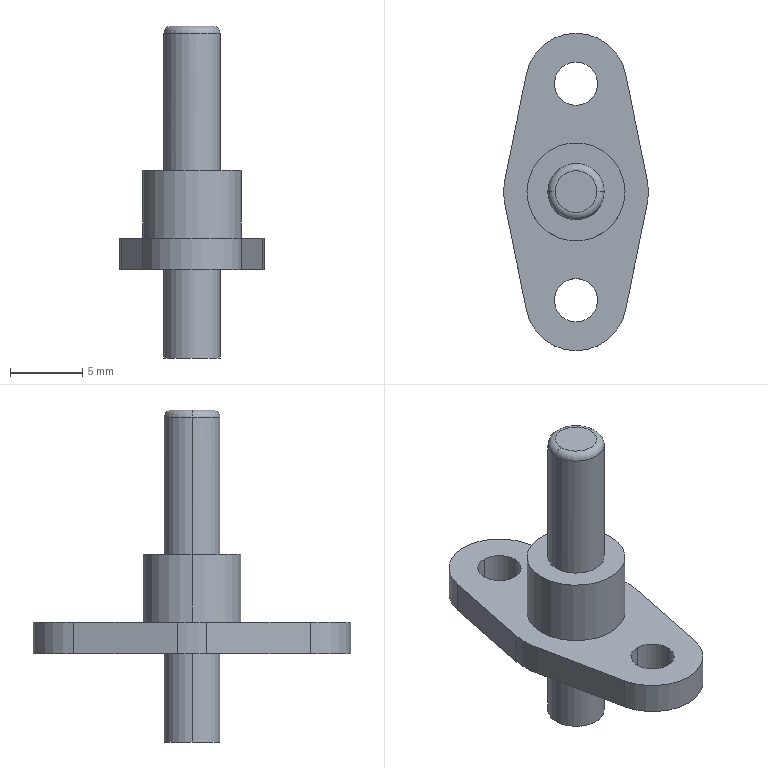Part | STEP file | ZXW722-L-79-1 | 1 solid | 30 faces | box 10 x 22 x 23 mm | volume 593.01 mm3 | cylinder 16 | plane 10 | torus 4 | commonest cylinder face diameters 3 x4 3.9 x4 2.5 x2 6.8 x2 7 x2 10 x2
STEP:
#1=CARTESIAN_POINT('',(0.,0.,0.));
#2=DIRECTION('',(0.,0.,1.));
#3=DIRECTION('',(1.,0.,0.));
#4=AXIS2_PLACEMENT_3D('',#1,#2,#3);
#5=CARTESIAN_POINT('',(1.45,0.,0.));
#6=VERTEX_POINT('',#5);
#7=CARTESIAN_POINT('',(-1.45,0.,0.));
#8=VERTEX_POINT('',#7);
#9=CARTESIAN_POINT('',(0.,0.,0.));
#10=DIRECTION('',(0.,0.,-1.));
#11=DIRECTION('',(1.,0.,0.));
#12=AXIS2_PLACEMENT_3D('',#9,#10,#11);
#13=CIRCLE('',#12,1.45);
#14=EDGE_CURVE('',#6,#8,#13,.T.);
#15=ORIENTED_EDGE('',*,*,#14,.T.);
#16=CARTESIAN_POINT('',(0.,0.,0.));
#17=DIRECTION('',(0.,0.,-1.));
#18=DIRECTION('',(-1.,0.,0.));
#19=AXIS2_PLACEMENT_3D('',#16,#17,#18);
#20=CIRCLE('',#19,1.45);
#21=EDGE_CURVE('',#8,#6,#20,.T.);
#22=ORIENTED_EDGE('',*,*,#21,.T.);
#23=EDGE_LOOP('',(#15,#22));
#24=FACE_OUTER_BOUND('',#23,.F.);
#25=CARTESIAN_POINT('',(0.,0.,0.));
#26=DIRECTION('',(0.,0.,1.));
#27=DIRECTION('',(-1.,0.,0.));
#28=AXIS2_PLACEMENT_3D('',#25,#26,#27);
#29=PLANE('',#28);
#30=ADVANCED_FACE('',(#24),#29,.T.);
#31=CARTESIAN_POINT('',(1.95,0.,-0.5));
#32=VERTEX_POINT('',#31);
#33=CARTESIAN_POINT('',(-1.95,-0.03686,-0.5));
#34=VERTEX_POINT('',#33);
#35=CARTESIAN_POINT('',(0.,0.,-0.5));
#36=DIRECTION('',(0.,0.,-1.));
#37=DIRECTION('',(1.,0.,0.));
#38=AXIS2_PLACEMENT_3D('',#35,#36,#37);
#39=CIRCLE('',#38,1.95);
#40=EDGE_CURVE('',#32,#34,#39,.T.);
#41=ORIENTED_EDGE('',*,*,#40,.T.);
#42=CARTESIAN_POINT('',(-1.95,0.,-0.5));
#43=VERTEX_POINT('',#42);
#44=CARTESIAN_POINT('',(0.,0.,-0.5));
#45=DIRECTION('',(0.,0.,-1.));
#46=DIRECTION('',(-0.9998,-0.0189,0.));
#47=AXIS2_PLACEMENT_3D('',#44,#45,#46);
#48=CIRCLE('',#47,1.95);
#49=EDGE_CURVE('',#34,#43,#48,.T.);
#50=ORIENTED_EDGE('',*,*,#49,.T.);
#51=CARTESIAN_POINT('',(-1.45,0.,-0.5));
#52=DIRECTION('',(0.,-1.,0.));
#53=DIRECTION('',(0.,0.,1.));
#54=AXIS2_PLACEMENT_3D('',#51,#52,#53);
#55=CIRCLE('',#54,0.5);
#56=EDGE_CURVE('',#8,#43,#55,.T.);
#57=ORIENTED_EDGE('',*,*,#56,.F.);
#58=ORIENTED_EDGE('',*,*,#14,.F.);
#59=CARTESIAN_POINT('',(1.45,0.,-0.5));
#60=DIRECTION('',(0.,1.,0.));
#61=DIRECTION('',(0.,0.,1.));
#62=AXIS2_PLACEMENT_3D('',#59,#60,#61);
#63=CIRCLE('',#62,0.5);
#64=EDGE_CURVE('',#6,#32,#63,.T.);
#65=ORIENTED_EDGE('',*,*,#64,.T.);
#66=EDGE_LOOP('',(#41,#50,#57,#58,#65));
#67=FACE_OUTER_BOUND('',#66,.F.);
#68=CARTESIAN_POINT('',(0.,0.,-0.5));
#69=DIRECTION('',(0.,0.,1.));
#70=DIRECTION('',(0.9998,0.0189,0.));
#71=AXIS2_PLACEMENT_3D('',#68,#69,#70);
#72=TOROIDAL_SURFACE('',#71,1.45,0.5);
#73=ADVANCED_FACE('',(#67),#72,.T.);
#74=ORIENTED_EDGE('',*,*,#49,.F.);
#75=ORIENTED_EDGE('',*,*,#40,.F.);
#76=CARTESIAN_POINT('',(1.95,0.,-10.));
#77=VERTEX_POINT('',#76);
#78=CARTESIAN_POINT('',(1.95,0.,-10.));
#79=DIRECTION('',(0.,0.,1.));
#80=VECTOR('',#79,9.5);
#81=LINE('',#78,#80);
#82=EDGE_CURVE('',#77,#32,#81,.T.);
#83=ORIENTED_EDGE('',*,*,#82,.F.);
#84=CARTESIAN_POINT('',(-1.95,0.,-10.));
#85=VERTEX_POINT('',#84);
#86=CARTESIAN_POINT('',(0.,0.,-10.));
#87=DIRECTION('',(0.,0.,1.));
#88=DIRECTION('',(-1.,0.,0.));
#89=AXIS2_PLACEMENT_3D('',#86,#87,#88);
#90=CIRCLE('',#89,1.95);
#91=EDGE_CURVE('',#85,#77,#90,.T.);
#92=ORIENTED_EDGE('',*,*,#91,.F.);
#93=CARTESIAN_POINT('',(-1.95,0.,-10.));
#94=DIRECTION('',(0.,0.,1.));
#95=VECTOR('',#94,9.5);
#96=LINE('',#93,#95);
#97=EDGE_CURVE('',#85,#43,#96,.T.);
#98=ORIENTED_EDGE('',*,*,#97,.T.);
#99=EDGE_LOOP('',(#74,#75,#83,#92,#98));
#100=FACE_OUTER_BOUND('',#99,.F.);
#101=CARTESIAN_POINT('',(0.,0.,-24.15));
#102=DIRECTION('',(0.,0.,1.));
#103=DIRECTION('',(-1.,0.,0.));
#104=AXIS2_PLACEMENT_3D('',#101,#102,#103);
#105=CYLINDRICAL_SURFACE('',#104,1.95);
#106=ADVANCED_FACE('',(#100),#105,.T.);
#107=CARTESIAN_POINT('',(1.95,0.03686,-0.5));
#108=VERTEX_POINT('',#107);
#109=CARTESIAN_POINT('',(0.,0.,-0.5));
#110=DIRECTION('',(0.,0.,-1.));
#111=DIRECTION('',(0.9998,0.0189,0.));
#112=AXIS2_PLACEMENT_3D('',#109,#110,#111);
#113=CIRCLE('',#112,1.95);
#114=EDGE_CURVE('',#108,#32,#113,.T.);
#115=ORIENTED_EDGE('',*,*,#114,.F.);
#116=CARTESIAN_POINT('',(0.,0.,-0.5));
#117=DIRECTION('',(0.,0.,-1.));
#118=DIRECTION('',(-1.,0.,0.));
#119=AXIS2_PLACEMENT_3D('',#116,#117,#118);
#120=CIRCLE('',#119,1.95);
#121=EDGE_CURVE('',#43,#108,#120,.T.);
#122=ORIENTED_EDGE('',*,*,#121,.F.);
#123=ORIENTED_EDGE('',*,*,#97,.F.);
#124=CARTESIAN_POINT('',(0.,0.,-10.));
#125=DIRECTION('',(0.,0.,1.));
#126=DIRECTION('',(1.,0.,0.));
#127=AXIS2_PLACEMENT_3D('',#124,#125,#126);
#128=CIRCLE('',#127,1.95);
#129=EDGE_CURVE('',#77,#85,#128,.T.);
#130=ORIENTED_EDGE('',*,*,#129,.F.);
#131=ORIENTED_EDGE('',*,*,#82,.T.);
#132=EDGE_LOOP('',(#115,#122,#123,#130,#131));
#133=FACE_OUTER_BOUND('',#132,.F.);
#134=CARTESIAN_POINT('',(0.,0.,-24.15));
#135=DIRECTION('',(0.,0.,1.));
#136=DIRECTION('',(-1.,0.,0.));
#137=AXIS2_PLACEMENT_3D('',#134,#135,#136);
#138=CYLINDRICAL_SURFACE('',#137,1.95);
#139=ADVANCED_FACE('',(#133),#138,.T.);
#140=ORIENTED_EDGE('',*,*,#121,.T.);
#141=ORIENTED_EDGE('',*,*,#114,.T.);
#142=ORIENTED_EDGE('',*,*,#64,.F.);
#143=ORIENTED_EDGE('',*,*,#21,.F.);
#144=ORIENTED_EDGE('',*,*,#56,.T.);
#145=EDGE_LOOP('',(#140,#141,#142,#143,#144));
#146=FACE_OUTER_BOUND('',#145,.F.);
#147=CARTESIAN_POINT('',(0.,0.,-0.5));
#148=DIRECTION('',(0.,0.,1.));
#149=DIRECTION('',(-0.9998,-0.0189,0.));
#150=AXIS2_PLACEMENT_3D('',#147,#148,#149);
#151=TOROIDAL_SURFACE('',#150,1.45,0.5);
#152=ADVANCED_FACE('',(#146),#151,.T.);
#153=CARTESIAN_POINT('',(-3.4,0.,-10.));
#154=VERTEX_POINT('',#153);
#155=CARTESIAN_POINT('',(3.4,0.,-10.));
#156=VERTEX_POINT('',#155);
#157=CARTESIAN_POINT('',(0.,0.,-10.));
#158=DIRECTION('',(0.,0.,-1.));
#159=DIRECTION('',(-1.,0.,0.));
#160=AXIS2_PLACEMENT_3D('',#157,#158,#159);
#161=CIRCLE('',#160,3.4);
#162=EDGE_CURVE('',#154,#156,#161,.T.);
#163=ORIENTED_EDGE('',*,*,#162,.T.);
#164=CARTESIAN_POINT('',(0.,0.,-10.));
#165=DIRECTION('',(0.,0.,-1.));
#166=DIRECTION('',(1.,0.,0.));
#167=AXIS2_PLACEMENT_3D('',#164,#165,#166);
#168=CIRCLE('',#167,3.4);
#169=EDGE_CURVE('',#156,#154,#168,.T.);
#170=ORIENTED_EDGE('',*,*,#169,.T.);
#171=EDGE_LOOP('',(#163,#170));
#172=FACE_OUTER_BOUND('',#171,.F.);
#173=ORIENTED_EDGE('',*,*,#91,.T.);
#174=ORIENTED_EDGE('',*,*,#129,.T.);
#175=EDGE_LOOP('',(#173,#174));
#176=FACE_BOUND('',#175,.F.);
#177=CARTESIAN_POINT('',(0.,0.,-10.));
#178=DIRECTION('',(0.,0.,1.));
#179=DIRECTION('',(-1.,0.,0.));
#180=AXIS2_PLACEMENT_3D('',#177,#178,#179);
#181=PLANE('',#180);
#182=ADVANCED_FACE('',(#172,#176),#181,.T.);
#183=CARTESIAN_POINT('',(3.4,0.,-14.7));
#184=VERTEX_POINT('',#183);
#185=CARTESIAN_POINT('',(-3.4,0.,-14.7));
#186=VERTEX_POINT('',#185);
#187=CARTESIAN_POINT('',(0.,0.,-14.7));
#188=DIRECTION('',(0.,0.,1.));
#189=DIRECTION('',(1.,0.,0.));
#190=AXIS2_PLACEMENT_3D('',#187,#188,#189);
#191=CIRCLE('',#190,3.4);
#192=EDGE_CURVE('',#184,#186,#191,.T.);
#193=ORIENTED_EDGE('',*,*,#192,.F.);
#194=CARTESIAN_POINT('',(3.4,0.,-14.7));
#195=DIRECTION('',(0.,0.,1.));
#196=VECTOR('',#195,4.7);
#197=LINE('',#194,#196);
#198=EDGE_CURVE('',#184,#156,#197,.T.);
#199=ORIENTED_EDGE('',*,*,#198,.T.);
#200=ORIENTED_EDGE('',*,*,#162,.F.);
#201=CARTESIAN_POINT('',(-3.4,0.,-14.7));
#202=DIRECTION('',(0.,0.,1.));
#203=VECTOR('',#202,4.7);
#204=LINE('',#201,#203);
#205=EDGE_CURVE('',#186,#154,#204,.T.);
#206=ORIENTED_EDGE('',*,*,#205,.F.);
#207=EDGE_LOOP('',(#193,#199,#200,#206));
#208=FACE_OUTER_BOUND('',#207,.F.);
#209=CARTESIAN_POINT('',(0.,0.,-24.15));
#210=DIRECTION('',(0.,0.,1.));
#211=DIRECTION('',(-1.,0.,0.));
#212=AXIS2_PLACEMENT_3D('',#209,#210,#211);
#213=CYLINDRICAL_SURFACE('',#212,3.4);
#214=ADVANCED_FACE('',(#208),#213,.T.);
#215=CARTESIAN_POINT('',(4.899,1.,-14.7));
#216=VERTEX_POINT('',#215);
#217=CARTESIAN_POINT('',(4.899,-1.,-14.7));
#218=VERTEX_POINT('',#217);
#219=CARTESIAN_POINT('',(0.,0.,-14.7));
#220=DIRECTION('',(0.,0.,-1.));
#221=DIRECTION('',(0.9798,0.2,0.));
#222=AXIS2_PLACEMENT_3D('',#219,#220,#221);
#223=CIRCLE('',#222,5.);
#224=EDGE_CURVE('',#216,#218,#223,.T.);
#225=ORIENTED_EDGE('',*,*,#224,.T.);
#226=CARTESIAN_POINT('',(3.429,-8.2,-14.7));
#227=VERTEX_POINT('',#226);
#228=CARTESIAN_POINT('',(4.899,-1.,-14.7));
#229=DIRECTION('',(-0.2,-0.9798,0.));
#230=VECTOR('',#229,7.348);
#231=LINE('',#228,#230);
#232=EDGE_CURVE('',#218,#227,#231,.T.);
#233=ORIENTED_EDGE('',*,*,#232,.T.);
#234=CARTESIAN_POINT('',(0.,-11.,-14.7));
#235=VERTEX_POINT('',#234);
#236=CARTESIAN_POINT('',(0.,-7.5,-14.7));
#237=DIRECTION('',(0.,0.,-1.));
#238=DIRECTION('',(0.9798,-0.2,0.));
#239=AXIS2_PLACEMENT_3D('',#236,#237,#238);
#240=CIRCLE('',#239,3.5);
#241=EDGE_CURVE('',#227,#235,#240,.T.);
#242=ORIENTED_EDGE('',*,*,#241,.T.);
#243=CARTESIAN_POINT('',(-3.429,-8.2,-14.7));
#244=VERTEX_POINT('',#243);
#245=CARTESIAN_POINT('',(0.,-7.5,-14.7));
#246=DIRECTION('',(0.,0.,-1.));
#247=DIRECTION('',(0.,-1.,0.));
#248=AXIS2_PLACEMENT_3D('',#245,#246,#247);
#249=CIRCLE('',#248,3.5);
#250=EDGE_CURVE('',#235,#244,#249,.T.);
#251=ORIENTED_EDGE('',*,*,#250,.T.);
#252=CARTESIAN_POINT('',(-4.899,-1.,-14.7));
#253=VERTEX_POINT('',#252);
#254=CARTESIAN_POINT('',(-3.429,-8.2,-14.7));
#255=DIRECTION('',(-0.2,0.9798,0.));
#256=VECTOR('',#255,7.348);
#257=LINE('',#254,#256);
#258=EDGE_CURVE('',#244,#253,#257,.T.);
#259=ORIENTED_EDGE('',*,*,#258,.T.);
#260=CARTESIAN_POINT('',(-4.899,1.,-14.7));
#261=VERTEX_POINT('',#260);
#262=CARTESIAN_POINT('',(0.,0.,-14.7));
#263=DIRECTION('',(0.,0.,-1.));
#264=DIRECTION('',(-0.9798,-0.2,0.));
#265=AXIS2_PLACEMENT_3D('',#262,#263,#264);
#266=CIRCLE('',#265,5.);
#267=EDGE_CURVE('',#253,#261,#266,.T.);
#268=ORIENTED_EDGE('',*,*,#267,.T.);
#269=CARTESIAN_POINT('',(-3.429,8.2,-14.7));
#270=VERTEX_POINT('',#269);
#271=CARTESIAN_POINT('',(-4.899,1.,-14.7));
#272=DIRECTION('',(0.2,0.9798,0.));
#273=VECTOR('',#272,7.348);
#274=LINE('',#271,#273);
#275=EDGE_CURVE('',#261,#270,#274,.T.);
#276=ORIENTED_EDGE('',*,*,#275,.T.);
#277=CARTESIAN_POINT('',(0.,11.,-14.7));
#278=VERTEX_POINT('',#277);
#279=CARTESIAN_POINT('',(0.,7.5,-14.7));
#280=DIRECTION('',(0.,0.,-1.));
#281=DIRECTION('',(-0.9798,0.2,0.));
#282=AXIS2_PLACEMENT_3D('',#279,#280,#281);
#283=CIRCLE('',#282,3.5);
#284=EDGE_CURVE('',#270,#278,#283,.T.);
#285=ORIENTED_EDGE('',*,*,#284,.T.);
#286=CARTESIAN_POINT('',(3.429,8.2,-14.7));
#287=VERTEX_POINT('',#286);
#288=CARTESIAN_POINT('',(0.,7.5,-14.7));
#289=DIRECTION('',(0.,0.,-1.));
#290=DIRECTION('',(0.,1.,0.));
#291=AXIS2_PLACEMENT_3D('',#288,#289,#290);
#292=CIRCLE('',#291,3.5);
#293=EDGE_CURVE('',#278,#287,#292,.T.);
#294=ORIENTED_EDGE('',*,*,#293,.T.);
#295=CARTESIAN_POINT('',(3.429,8.2,-14.7));
#296=DIRECTION('',(0.2,-0.9798,0.));
#297=VECTOR('',#296,7.348);
#298=LINE('',#295,#297);
#299=EDGE_CURVE('',#287,#216,#298,.T.);
#300=ORIENTED_EDGE('',*,*,#299,.T.);
#301=EDGE_LOOP('',(#225,#233,#242,#251,#259,#268,#276,#285,#294,#300));
#302=FACE_OUTER_BOUND('',#301,.F.);
#303=CARTESIAN_POINT('',(0.,-6.,-14.7));
#304=VERTEX_POINT('',#303);
#305=CARTESIAN_POINT('',(0.,-9.,-14.7));
#306=VERTEX_POINT('',#305);
#307=CARTESIAN_POINT('',(0.,-7.5,-14.7));
#308=DIRECTION('',(0.,0.,1.));
#309=DIRECTION('',(0.,1.,0.));
#310=AXIS2_PLACEMENT_3D('',#307,#308,#309);
#311=CIRCLE('',#310,1.5);
#312=EDGE_CURVE('',#304,#306,#311,.T.);
#313=ORIENTED_EDGE('',*,*,#312,.T.);
#314=CARTESIAN_POINT('',(0.,-7.5,-14.7));
#315=DIRECTION('',(0.,0.,1.));
#316=DIRECTION('',(0.,-1.,0.));
#317=AXIS2_PLACEMENT_3D('',#314,#315,#316);
#318=CIRCLE('',#317,1.5);
#319=EDGE_CURVE('',#306,#304,#318,.T.);
#320=ORIENTED_EDGE('',*,*,#319,.T.);
#321=EDGE_LOOP('',(#313,#320));
#322=FACE_BOUND('',#321,.F.);
#323=CARTESIAN_POINT('',(0.,9.,-14.7));
#324=VERTEX_POINT('',#323);
#325=CARTESIAN_POINT('',(0.,6.,-14.7));
#326=VERTEX_POINT('',#325);
#327=CARTESIAN_POINT('',(0.,7.5,-14.7));
#328=DIRECTION('',(0.,0.,1.));
#329=DIRECTION('',(0.,1.,0.));
#330=AXIS2_PLACEMENT_3D('',#327,#328,#329);
#331=CIRCLE('',#330,1.5);
#332=EDGE_CURVE('',#324,#326,#331,.T.);
#333=ORIENTED_EDGE('',*,*,#332,.T.);
#334=CARTESIAN_POINT('',(0.,7.5,-14.7));
#335=DIRECTION('',(0.,0.,1.));
#336=DIRECTION('',(0.,-1.,0.));
#337=AXIS2_PLACEMENT_3D('',#334,#335,#336);
#338=CIRCLE('',#337,1.5);
#339=EDGE_CURVE('',#326,#324,#338,.T.);
#340=ORIENTED_EDGE('',*,*,#339,.T.);
#341=EDGE_LOOP('',(#333,#340));
#342=FACE_BOUND('',#341,.F.);
#343=ORIENTED_EDGE('',*,*,#192,.T.);
#344=CARTESIAN_POINT('',(0.,0.,-14.7));
#345=DIRECTION('',(0.,0.,1.));
#346=DIRECTION('',(-1.,0.,0.));
#347=AXIS2_PLACEMENT_3D('',#344,#345,#346);
#348=CIRCLE('',#347,3.4);
#349=EDGE_CURVE('',#186,#184,#348,.T.);
#350=ORIENTED_EDGE('',*,*,#349,.T.);
#351=EDGE_LOOP('',(#343,#350));
#352=FACE_BOUND('',#351,.F.);
#353=CARTESIAN_POINT('',(0.,0.,-14.7));
#354=DIRECTION('',(0.,0.,-1.));
#355=DIRECTION('',(0.,1.,0.));
#356=AXIS2_PLACEMENT_3D('',#353,#354,#355);
#357=PLANE('',#356);
#358=ADVANCED_FACE('',(#302,#322,#342,#352),#357,.F.);
#359=ORIENTED_EDGE('',*,*,#224,.F.);
#360=CARTESIAN_POINT('',(4.899,1.,-16.9));
#361=VERTEX_POINT('',#360);
#362=CARTESIAN_POINT('',(4.899,1.,-14.7));
#363=DIRECTION('',(0.,0.,-1.));
#364=VECTOR('',#363,2.2);
#365=LINE('',#362,#364);
#366=EDGE_CURVE('',#216,#361,#365,.T.);
#367=ORIENTED_EDGE('',*,*,#366,.T.);
#368=CARTESIAN_POINT('',(4.899,-1.,-16.9));
#369=VERTEX_POINT('',#368);
#370=CARTESIAN_POINT('',(0.,0.,-16.9));
#371=DIRECTION('',(0.,0.,1.));
#372=DIRECTION('',(0.9798,-0.2,0.));
#373=AXIS2_PLACEMENT_3D('',#370,#371,#372);
#374=CIRCLE('',#373,5.);
#375=EDGE_CURVE('',#369,#361,#374,.T.);
#376=ORIENTED_EDGE('',*,*,#375,.F.);
#377=CARTESIAN_POINT('',(4.899,-1.,-16.9));
#378=DIRECTION('',(0.,0.,1.));
#379=VECTOR('',#378,2.2);
#380=LINE('',#377,#379);
#381=EDGE_CURVE('',#369,#218,#380,.T.);
#382=ORIENTED_EDGE('',*,*,#381,.T.);
#383=EDGE_LOOP('',(#359,#367,#376,#382));
#384=FACE_OUTER_BOUND('',#383,.F.);
#385=CARTESIAN_POINT('',(0.,0.,-14.7));
#386=DIRECTION('',(0.,0.,-1.));
#387=DIRECTION('',(0.,1.,0.));
#388=AXIS2_PLACEMENT_3D('',#385,#386,#387);
#389=CYLINDRICAL_SURFACE('',#388,5.);
#390=ADVANCED_FACE('',(#384),#389,.T.);
#391=ORIENTED_EDGE('',*,*,#299,.F.);
#392=CARTESIAN_POINT('',(3.429,8.2,-16.9));
#393=VERTEX_POINT('',#392);
#394=CARTESIAN_POINT('',(3.429,8.2,-16.9));
#395=DIRECTION('',(0.,0.,1.));
#396=VECTOR('',#395,2.2);
#397=LINE('',#394,#396);
#398=EDGE_CURVE('',#393,#287,#397,.T.);
#399=ORIENTED_EDGE('',*,*,#398,.F.);
#400=CARTESIAN_POINT('',(4.899,1.,-16.9));
#401=DIRECTION('',(-0.2,0.9798,0.));
#402=VECTOR('',#401,7.348);
#403=LINE('',#400,#402);
#404=EDGE_CURVE('',#361,#393,#403,.T.);
#405=ORIENTED_EDGE('',*,*,#404,.F.);
#406=ORIENTED_EDGE('',*,*,#366,.F.);
#407=EDGE_LOOP('',(#391,#399,#405,#406));
#408=FACE_OUTER_BOUND('',#407,.F.);
#409=CARTESIAN_POINT('',(3.429,8.2,-14.7));
#410=DIRECTION('',(0.9798,0.2,0.));
#411=DIRECTION('',(0.2,-0.9798,0.));
#412=AXIS2_PLACEMENT_3D('',#409,#410,#411);
#413=PLANE('',#412);
#414=ADVANCED_FACE('',(#408),#413,.T.);
#415=ORIENTED_EDGE('',*,*,#293,.F.);
#416=ORIENTED_EDGE('',*,*,#284,.F.);
#417=CARTESIAN_POINT('',(-3.429,8.2,-16.9));
#418=VERTEX_POINT('',#417);
#419=CARTESIAN_POINT('',(-3.429,8.2,-14.7));
#420=DIRECTION('',(0.,0.,-1.));
#421=VECTOR('',#420,2.2);
#422=LINE('',#419,#421);
#423=EDGE_CURVE('',#270,#418,#422,.T.);
#424=ORIENTED_EDGE('',*,*,#423,.T.);
#425=CARTESIAN_POINT('',(0.,11.,-16.9));
#426=VERTEX_POINT('',#425);
#427=CARTESIAN_POINT('',(0.,7.5,-16.9));
#428=DIRECTION('',(0.,0.,1.));
#429=DIRECTION('',(0.,1.,0.));
#430=AXIS2_PLACEMENT_3D('',#427,#428,#429);
#431=CIRCLE('',#430,3.5);
#432=EDGE_CURVE('',#426,#418,#431,.T.);
#433=ORIENTED_EDGE('',*,*,#432,.F.);
#434=CARTESIAN_POINT('',(0.,7.5,-16.9));
#435=DIRECTION('',(0.,0.,1.));
#436=DIRECTION('',(0.9798,0.2,0.));
#437=AXIS2_PLACEMENT_3D('',#434,#435,#436);
#438=CIRCLE('',#437,3.5);
#439=EDGE_CURVE('',#393,#426,#438,.T.);
#440=ORIENTED_EDGE('',*,*,#439,.F.);
#441=ORIENTED_EDGE('',*,*,#398,.T.);
#442=EDGE_LOOP('',(#415,#416,#424,#433,#440,#441));
#443=FACE_OUTER_BOUND('',#442,.F.);
#444=CARTESIAN_POINT('',(0.,7.5,-14.7));
#445=DIRECTION('',(0.,0.,-1.));
#446=DIRECTION('',(0.,1.,0.));
#447=AXIS2_PLACEMENT_3D('',#444,#445,#446);
#448=CYLINDRICAL_SURFACE('',#447,3.5);
#449=ADVANCED_FACE('',(#443),#448,.T.);
#450=ORIENTED_EDGE('',*,*,#275,.F.);
#451=CARTESIAN_POINT('',(-4.899,1.,-16.9));
#452=VERTEX_POINT('',#451);
#453=CARTESIAN_POINT('',(-4.899,1.,-16.9));
#454=DIRECTION('',(0.,0.,1.));
#455=VECTOR('',#454,2.2);
#456=LINE('',#453,#455);
#457=EDGE_CURVE('',#452,#261,#456,.T.);
#458=ORIENTED_EDGE('',*,*,#457,.F.);
#459=CARTESIAN_POINT('',(-3.429,8.2,-16.9));
#460=DIRECTION('',(-0.2,-0.9798,0.));
#461=VECTOR('',#460,7.348);
#462=LINE('',#459,#461);
#463=EDGE_CURVE('',#418,#452,#462,.T.);
#464=ORIENTED_EDGE('',*,*,#463,.F.);
#465=ORIENTED_EDGE('',*,*,#423,.F.);
#466=EDGE_LOOP('',(#450,#458,#464,#465));
#467=FACE_OUTER_BOUND('',#466,.F.);
#468=CARTESIAN_POINT('',(-4.899,1.,-14.7));
#469=DIRECTION('',(-0.9798,0.2,0.));
#470=DIRECTION('',(0.2,0.9798,0.));
#471=AXIS2_PLACEMENT_3D('',#468,#469,#470);
#472=PLANE('',#471);
#473=ADVANCED_FACE('',(#467),#472,.T.);
#474=ORIENTED_EDGE('',*,*,#267,.F.);
#475=CARTESIAN_POINT('',(-4.899,-1.,-16.9));
#476=VERTEX_POINT('',#475);
#477=CARTESIAN_POINT('',(-4.899,-1.,-14.7));
#478=DIRECTION('',(0.,0.,-1.));
#479=VECTOR('',#478,2.2);
#480=LINE('',#477,#479);
#481=EDGE_CURVE('',#253,#476,#480,.T.);
#482=ORIENTED_EDGE('',*,*,#481,.T.);
#483=CARTESIAN_POINT('',(0.,0.,-16.9));
#484=DIRECTION('',(0.,0.,1.));
#485=DIRECTION('',(-0.9798,0.2,0.));
#486=AXIS2_PLACEMENT_3D('',#483,#484,#485);
#487=CIRCLE('',#486,5.);
#488=EDGE_CURVE('',#452,#476,#487,.T.);
#489=ORIENTED_EDGE('',*,*,#488,.F.);
#490=ORIENTED_EDGE('',*,*,#457,.T.);
#491=EDGE_LOOP('',(#474,#482,#489,#490));
#492=FACE_OUTER_BOUND('',#491,.F.);
#493=CARTESIAN_POINT('',(0.,0.,-14.7));
#494=DIRECTION('',(0.,0.,-1.));
#495=DIRECTION('',(0.,1.,0.));
#496=AXIS2_PLACEMENT_3D('',#493,#494,#495);
#497=CYLINDRICAL_SURFACE('',#496,5.);
#498=ADVANCED_FACE('',(#492),#497,.T.);
#499=ORIENTED_EDGE('',*,*,#258,.F.);
#500=CARTESIAN_POINT('',(-3.429,-8.2,-16.9));
#501=VERTEX_POINT('',#500);
#502=CARTESIAN_POINT('',(-3.429,-8.2,-16.9));
#503=DIRECTION('',(0.,0.,1.));
#504=VECTOR('',#503,2.2);
#505=LINE('',#502,#504);
#506=EDGE_CURVE('',#501,#244,#505,.T.);
#507=ORIENTED_EDGE('',*,*,#506,.F.);
#508=CARTESIAN_POINT('',(-4.899,-1.,-16.9));
#509=DIRECTION('',(0.2,-0.9798,0.));
#510=VECTOR('',#509,7.348);
#511=LINE('',#508,#510);
#512=EDGE_CURVE('',#476,#501,#511,.T.);
#513=ORIENTED_EDGE('',*,*,#512,.F.);
#514=ORIENTED_EDGE('',*,*,#481,.F.);
#515=EDGE_LOOP('',(#499,#507,#513,#514));
#516=FACE_OUTER_BOUND('',#515,.F.);
#517=CARTESIAN_POINT('',(-3.429,-8.2,-14.7));
#518=DIRECTION('',(-0.9798,-0.2,0.));
#519=DIRECTION('',(-0.2,0.9798,0.));
#520=AXIS2_PLACEMENT_3D('',#517,#518,#519);
#521=PLANE('',#520);
#522=ADVANCED_FACE('',(#516),#521,.T.);
#523=ORIENTED_EDGE('',*,*,#250,.F.);
#524=ORIENTED_EDGE('',*,*,#241,.F.);
#525=CARTESIAN_POINT('',(3.429,-8.2,-16.9));
#526=VERTEX_POINT('',#525);
#527=CARTESIAN_POINT('',(3.429,-8.2,-14.7));
#528=DIRECTION('',(0.,0.,-1.));
#529=VECTOR('',#528,2.2);
#530=LINE('',#527,#529);
#531=EDGE_CURVE('',#227,#526,#530,.T.);
#532=ORIENTED_EDGE('',*,*,#531,.T.);
#533=CARTESIAN_POINT('',(0.,-11.,-16.9));
#534=VERTEX_POINT('',#533);
#535=CARTESIAN_POINT('',(0.,-7.5,-16.9));
#536=DIRECTION('',(0.,0.,1.));
#537=DIRECTION('',(0.,-1.,0.));
#538=AXIS2_PLACEMENT_3D('',#535,#536,#537);
#539=CIRCLE('',#538,3.5);
#540=EDGE_CURVE('',#534,#526,#539,.T.);
#541=ORIENTED_EDGE('',*,*,#540,.F.);
#542=CARTESIAN_POINT('',(0.,-7.5,-16.9));
#543=DIRECTION('',(0.,0.,1.));
#544=DIRECTION('',(-0.9798,-0.2,0.));
#545=AXIS2_PLACEMENT_3D('',#542,#543,#544);
#546=CIRCLE('',#545,3.5);
#547=EDGE_CURVE('',#501,#534,#546,.T.);
#548=ORIENTED_EDGE('',*,*,#547,.F.);
#549=ORIENTED_EDGE('',*,*,#506,.T.);
#550=EDGE_LOOP('',(#523,#524,#532,#541,#548,#549));
#551=FACE_OUTER_BOUND('',#550,.F.);
#552=CARTESIAN_POINT('',(0.,-7.5,-14.7));
#553=DIRECTION('',(0.,0.,-1.));
#554=DIRECTION('',(0.,1.,0.));
#555=AXIS2_PLACEMENT_3D('',#552,#553,#554);
#556=CYLINDRICAL_SURFACE('',#555,3.5);
#557=ADVANCED_FACE('',(#551),#556,.T.);
#558=ORIENTED_EDGE('',*,*,#232,.F.);
#559=ORIENTED_EDGE('',*,*,#381,.F.);
#560=CARTESIAN_POINT('',(3.429,-8.2,-16.9));
#561=DIRECTION('',(0.2,0.9798,0.));
#562=VECTOR('',#561,7.348);
#563=LINE('',#560,#562);
#564=EDGE_CURVE('',#526,#369,#563,.T.);
#565=ORIENTED_EDGE('',*,*,#564,.F.);
#566=ORIENTED_EDGE('',*,*,#531,.F.);
#567=EDGE_LOOP('',(#558,#559,#565,#566));
#568=FACE_OUTER_BOUND('',#567,.F.);
#569=CARTESIAN_POINT('',(4.899,-1.,-14.7));
#570=DIRECTION('',(0.9798,-0.2,0.));
#571=DIRECTION('',(-0.2,-0.9798,0.));
#572=AXIS2_PLACEMENT_3D('',#569,#570,#571);
#573=PLANE('',#572);
#574=ADVANCED_FACE('',(#568),#573,.T.);
#575=ORIENTED_EDGE('',*,*,#375,.T.);
#576=ORIENTED_EDGE('',*,*,#404,.T.);
#577=ORIENTED_EDGE('',*,*,#439,.T.);
#578=ORIENTED_EDGE('',*,*,#432,.T.);
#579=ORIENTED_EDGE('',*,*,#463,.T.);
#580=ORIENTED_EDGE('',*,*,#488,.T.);
#581=ORIENTED_EDGE('',*,*,#512,.T.);
#582=ORIENTED_EDGE('',*,*,#547,.T.);
#583=ORIENTED_EDGE('',*,*,#540,.T.);
#584=ORIENTED_EDGE('',*,*,#564,.T.);
#585=EDGE_LOOP('',(#575,#576,#577,#578,#579,#580,#581,#582,#583,#584));
#586=FACE_OUTER_BOUND('',#585,.F.);
#587=CARTESIAN_POINT('',(0.,-9.,-16.9));
#588=VERTEX_POINT('',#587);
#589=CARTESIAN_POINT('',(0.,-6.,-16.9));
#590=VERTEX_POINT('',#589);
#591=CARTESIAN_POINT('',(0.,-7.5,-16.9));
#592=DIRECTION('',(0.,0.,-1.));
#593=DIRECTION('',(0.,-1.,0.));
#594=AXIS2_PLACEMENT_3D('',#591,#592,#593);
#595=CIRCLE('',#594,1.5);
#596=EDGE_CURVE('',#588,#590,#595,.T.);
#597=ORIENTED_EDGE('',*,*,#596,.T.);
#598=CARTESIAN_POINT('',(0.,-7.5,-16.9));
#599=DIRECTION('',(0.,0.,-1.));
#600=DIRECTION('',(0.,1.,0.));
#601=AXIS2_PLACEMENT_3D('',#598,#599,#600);
#602=CIRCLE('',#601,1.5);
#603=EDGE_CURVE('',#590,#588,#602,.T.);
#604=ORIENTED_EDGE('',*,*,#603,.T.);
#605=EDGE_LOOP('',(#597,#604));
#606=FACE_BOUND('',#605,.F.);
#607=CARTESIAN_POINT('',(0.,6.,-16.9));
#608=VERTEX_POINT('',#607);
#609=CARTESIAN_POINT('',(0.,9.,-16.9));
#610=VERTEX_POINT('',#609);
#611=CARTESIAN_POINT('',(0.,7.5,-16.9));
#612=DIRECTION('',(0.,0.,-1.));
#613=DIRECTION('',(0.,-1.,0.));
#614=AXIS2_PLACEMENT_3D('',#611,#612,#613);
#615=CIRCLE('',#614,1.5);
#616=EDGE_CURVE('',#608,#610,#615,.T.);
#617=ORIENTED_EDGE('',*,*,#616,.T.);
#618=CARTESIAN_POINT('',(0.,7.5,-16.9));
#619=DIRECTION('',(0.,0.,-1.));
#620=DIRECTION('',(0.,1.,0.));
#621=AXIS2_PLACEMENT_3D('',#618,#619,#620);
#622=CIRCLE('',#621,1.5);
#623=EDGE_CURVE('',#610,#608,#622,.T.);
#624=ORIENTED_EDGE('',*,*,#623,.T.);
#625=EDGE_LOOP('',(#617,#624));
#626=FACE_BOUND('',#625,.F.);
#627=CARTESIAN_POINT('',(-1.95,0.,-16.9));
#628=VERTEX_POINT('',#627);
#629=CARTESIAN_POINT('',(1.95,0.,-16.9));
#630=VERTEX_POINT('',#629);
#631=CARTESIAN_POINT('',(0.,0.,-16.9));
#632=DIRECTION('',(0.,0.,-1.));
#633=DIRECTION('',(-1.,0.,0.));
#634=AXIS2_PLACEMENT_3D('',#631,#632,#633);
#635=CIRCLE('',#634,1.95);
#636=EDGE_CURVE('',#628,#630,#635,.T.);
#637=ORIENTED_EDGE('',*,*,#636,.T.);
#638=CARTESIAN_POINT('',(0.,0.,-16.9));
#639=DIRECTION('',(0.,0.,-1.));
#640=DIRECTION('',(1.,0.,0.));
#641=AXIS2_PLACEMENT_3D('',#638,#639,#640);
#642=CIRCLE('',#641,1.95);
#643=EDGE_CURVE('',#630,#628,#642,.T.);
#644=ORIENTED_EDGE('',*,*,#643,.T.);
#645=EDGE_LOOP('',(#637,#644));
#646=FACE_BOUND('',#645,.F.);
#647=CARTESIAN_POINT('',(0.,0.,-16.9));
#648=DIRECTION('',(0.,0.,-1.));
#649=DIRECTION('',(0.,1.,0.));
#650=AXIS2_PLACEMENT_3D('',#647,#648,#649);
#651=PLANE('',#650);
#652=ADVANCED_FACE('',(#586,#606,#626,#646),#651,.T.);
#653=ORIENTED_EDGE('',*,*,#312,.F.);
#654=CARTESIAN_POINT('',(0.,-6.,-16.9));
#655=DIRECTION('',(0.,0.,1.));
#656=VECTOR('',#655,2.2);
#657=LINE('',#654,#656);
#658=EDGE_CURVE('',#590,#304,#657,.T.);
#659=ORIENTED_EDGE('',*,*,#658,.F.);
#660=ORIENTED_EDGE('',*,*,#596,.F.);
#661=CARTESIAN_POINT('',(0.,-9.,-16.9));
#662=DIRECTION('',(0.,0.,1.));
#663=VECTOR('',#662,2.2);
#664=LINE('',#661,#663);
#665=EDGE_CURVE('',#588,#306,#664,.T.);
#666=ORIENTED_EDGE('',*,*,#665,.T.);
#667=EDGE_LOOP('',(#653,#659,#660,#666));
#668=FACE_OUTER_BOUND('',#667,.F.);
#669=CARTESIAN_POINT('',(0.,-7.5,-14.7));
#670=DIRECTION('',(0.,0.,-1.));
#671=DIRECTION('',(0.,1.,0.));
#672=AXIS2_PLACEMENT_3D('',#669,#670,#671);
#673=CYLINDRICAL_SURFACE('',#672,1.5);
#674=ADVANCED_FACE('',(#668),#673,.F.);
#675=ORIENTED_EDGE('',*,*,#319,.F.);
#676=ORIENTED_EDGE('',*,*,#665,.F.);
#677=ORIENTED_EDGE('',*,*,#603,.F.);
#678=ORIENTED_EDGE('',*,*,#658,.T.);
#679=EDGE_LOOP('',(#675,#676,#677,#678));
#680=FACE_OUTER_BOUND('',#679,.F.);
#681=CARTESIAN_POINT('',(0.,-7.5,-14.7));
#682=DIRECTION('',(0.,0.,-1.));
#683=DIRECTION('',(0.,1.,0.));
#684=AXIS2_PLACEMENT_3D('',#681,#682,#683);
#685=CYLINDRICAL_SURFACE('',#684,1.5);
#686=ADVANCED_FACE('',(#680),#685,.F.);
#687=ORIENTED_EDGE('',*,*,#332,.F.);
#688=CARTESIAN_POINT('',(0.,9.,-16.9));
#689=DIRECTION('',(0.,0.,1.));
#690=VECTOR('',#689,2.2);
#691=LINE('',#688,#690);
#692=EDGE_CURVE('',#610,#324,#691,.T.);
#693=ORIENTED_EDGE('',*,*,#692,.F.);
#694=ORIENTED_EDGE('',*,*,#616,.F.);
#695=CARTESIAN_POINT('',(0.,6.,-16.9));
#696=DIRECTION('',(0.,0.,1.));
#697=VECTOR('',#696,2.2);
#698=LINE('',#695,#697);
#699=EDGE_CURVE('',#608,#326,#698,.T.);
#700=ORIENTED_EDGE('',*,*,#699,.T.);
#701=EDGE_LOOP('',(#687,#693,#694,#700));
#702=FACE_OUTER_BOUND('',#701,.F.);
#703=CARTESIAN_POINT('',(0.,7.5,-14.7));
#704=DIRECTION('',(0.,0.,-1.));
#705=DIRECTION('',(0.,1.,0.));
#706=AXIS2_PLACEMENT_3D('',#703,#704,#705);
#707=CYLINDRICAL_SURFACE('',#706,1.5);
#708=ADVANCED_FACE('',(#702),#707,.F.);
#709=ORIENTED_EDGE('',*,*,#339,.F.);
#710=ORIENTED_EDGE('',*,*,#699,.F.);
#711=ORIENTED_EDGE('',*,*,#623,.F.);
#712=ORIENTED_EDGE('',*,*,#692,.T.);
#713=EDGE_LOOP('',(#709,#710,#711,#712));
#714=FACE_OUTER_BOUND('',#713,.F.);
#715=CARTESIAN_POINT('',(0.,7.5,-14.7));
#716=DIRECTION('',(0.,0.,-1.));
#717=DIRECTION('',(0.,1.,0.));
#718=AXIS2_PLACEMENT_3D('',#715,#716,#717);
#719=CYLINDRICAL_SURFACE('',#718,1.5);
#720=ADVANCED_FACE('',(#714),#719,.F.);
#721=ORIENTED_EDGE('',*,*,#636,.F.);
#722=CARTESIAN_POINT('',(-1.95,0.,-23.));
#723=VERTEX_POINT('',#722);
#724=CARTESIAN_POINT('',(-1.95,0.,-23.));
#725=DIRECTION('',(0.,0.,1.));
#726=VECTOR('',#725,6.1);
#727=LINE('',#724,#726);
#728=EDGE_CURVE('',#723,#628,#727,.T.);
#729=ORIENTED_EDGE('',*,*,#728,.F.);
#730=CARTESIAN_POINT('',(1.95,0.,-23.));
#731=VERTEX_POINT('',#730);
#732=CARTESIAN_POINT('',(0.,0.,-23.));
#733=DIRECTION('',(0.,0.,1.));
#734=DIRECTION('',(1.,0.,0.));
#735=AXIS2_PLACEMENT_3D('',#732,#733,#734);
#736=CIRCLE('',#735,1.95);
#737=EDGE_CURVE('',#731,#723,#736,.T.);
#738=ORIENTED_EDGE('',*,*,#737,.F.);
#739=CARTESIAN_POINT('',(1.95,0.,-23.));
#740=DIRECTION('',(0.,0.,1.));
#741=VECTOR('',#740,6.1);
#742=LINE('',#739,#741);
#743=EDGE_CURVE('',#731,#630,#742,.T.);
#744=ORIENTED_EDGE('',*,*,#743,.T.);
#745=EDGE_LOOP('',(#721,#729,#738,#744));
#746=FACE_OUTER_BOUND('',#745,.F.);
#747=CARTESIAN_POINT('',(0.,0.,-24.15));
#748=DIRECTION('',(0.,0.,1.));
#749=DIRECTION('',(-1.,0.,0.));
#750=AXIS2_PLACEMENT_3D('',#747,#748,#749);
#751=CYLINDRICAL_SURFACE('',#750,1.95);
#752=ADVANCED_FACE('',(#746),#751,.T.);
#753=ORIENTED_EDGE('',*,*,#643,.F.);
#754=ORIENTED_EDGE('',*,*,#743,.F.);
#755=CARTESIAN_POINT('',(0.,0.,-23.));
#756=DIRECTION('',(0.,0.,1.));
#757=DIRECTION('',(-1.,0.,0.));
#758=AXIS2_PLACEMENT_3D('',#755,#756,#757);
#759=CIRCLE('',#758,1.95);
#760=EDGE_CURVE('',#723,#731,#759,.T.);
#761=ORIENTED_EDGE('',*,*,#760,.F.);
#762=ORIENTED_EDGE('',*,*,#728,.T.);
#763=EDGE_LOOP('',(#753,#754,#761,#762));
#764=FACE_OUTER_BOUND('',#763,.F.);
#765=CARTESIAN_POINT('',(0.,0.,-24.15));
#766=DIRECTION('',(0.,0.,1.));
#767=DIRECTION('',(-1.,0.,0.));
#768=AXIS2_PLACEMENT_3D('',#765,#766,#767);
#769=CYLINDRICAL_SURFACE('',#768,1.95);
#770=ADVANCED_FACE('',(#764),#769,.T.);
#771=ORIENTED_EDGE('',*,*,#760,.T.);
#772=ORIENTED_EDGE('',*,*,#737,.T.);
#773=EDGE_LOOP('',(#771,#772));
#774=FACE_OUTER_BOUND('',#773,.F.);
#775=CARTESIAN_POINT('',(-1.25,0.,-23.));
#776=VERTEX_POINT('',#775);
#777=CARTESIAN_POINT('',(1.25,0.,-23.));
#778=VERTEX_POINT('',#777);
#779=CARTESIAN_POINT('',(0.,0.,-23.));
#780=DIRECTION('',(0.,0.,-1.));
#781=DIRECTION('',(-1.,0.,0.));
#782=AXIS2_PLACEMENT_3D('',#779,#780,#781);
#783=CIRCLE('',#782,1.25);
#784=EDGE_CURVE('',#776,#778,#783,.T.);
#785=ORIENTED_EDGE('',*,*,#784,.T.);
#786=CARTESIAN_POINT('',(0.,0.,-23.));
#787=DIRECTION('',(0.,0.,-1.));
#788=DIRECTION('',(1.,0.,0.));
#789=AXIS2_PLACEMENT_3D('',#786,#787,#788);
#790=CIRCLE('',#789,1.25);
#791=EDGE_CURVE('',#778,#776,#790,.T.);
#792=ORIENTED_EDGE('',*,*,#791,.T.);
#793=EDGE_LOOP('',(#785,#792));
#794=FACE_BOUND('',#793,.F.);
#795=CARTESIAN_POINT('',(0.,0.,-23.));
#796=DIRECTION('',(0.,0.,1.));
#797=DIRECTION('',(-1.,0.,0.));
#798=AXIS2_PLACEMENT_3D('',#795,#796,#797);
#799=PLANE('',#798);
#800=ADVANCED_FACE('',(#774,#794),#799,.F.);
#801=CARTESIAN_POINT('',(-1.249,0.03833,-1.2));
#802=VERTEX_POINT('',#801);
#803=CARTESIAN_POINT('',(-1.25,0.,-1.2));
#804=VERTEX_POINT('',#803);
#805=CARTESIAN_POINT('',(0.,0.,-1.2));
#806=DIRECTION('',(0.,0.,1.));
#807=DIRECTION('',(-0.9995,0.03066,0.));
#808=AXIS2_PLACEMENT_3D('',#805,#806,#807);
#809=CIRCLE('',#808,1.25);
#810=EDGE_CURVE('',#802,#804,#809,.T.);
#811=ORIENTED_EDGE('',*,*,#810,.F.);
#812=CARTESIAN_POINT('',(1.25,0.,-1.2));
#813=VERTEX_POINT('',#812);
#814=CARTESIAN_POINT('',(0.,0.,-1.2));
#815=DIRECTION('',(0.,0.,1.));
#816=DIRECTION('',(1.,0.,0.));
#817=AXIS2_PLACEMENT_3D('',#814,#815,#816);
#818=CIRCLE('',#817,1.25);
#819=EDGE_CURVE('',#813,#802,#818,.T.);
#820=ORIENTED_EDGE('',*,*,#819,.F.);
#821=CARTESIAN_POINT('',(1.25,0.,-1.2));
#822=DIRECTION('',(0.,0.,-1.));
#823=VECTOR('',#822,21.8);
#824=LINE('',#821,#823);
#825=EDGE_CURVE('',#813,#778,#824,.T.);
#826=ORIENTED_EDGE('',*,*,#825,.T.);
#827=ORIENTED_EDGE('',*,*,#784,.F.);
#828=CARTESIAN_POINT('',(-1.25,0.,-1.2));
#829=DIRECTION('',(0.,0.,-1.));
#830=VECTOR('',#829,21.8);
#831=LINE('',#828,#830);
#832=EDGE_CURVE('',#804,#776,#831,.T.);
#833=ORIENTED_EDGE('',*,*,#832,.F.);
#834=EDGE_LOOP('',(#811,#820,#826,#827,#833));
#835=FACE_OUTER_BOUND('',#834,.F.);
#836=CARTESIAN_POINT('',(0.,0.,-24.15));
#837=DIRECTION('',(0.,0.,1.));
#838=DIRECTION('',(-1.,0.,0.));
#839=AXIS2_PLACEMENT_3D('',#836,#837,#838);
#840=CYLINDRICAL_SURFACE('',#839,1.25);
#841=ADVANCED_FACE('',(#835),#840,.F.);
#842=CARTESIAN_POINT('',(0.75,0.,-0.7));
#843=VERTEX_POINT('',#842);
#844=CARTESIAN_POINT('',(-0.75,0.,-0.7));
#845=VERTEX_POINT('',#844);
#846=CARTESIAN_POINT('',(0.,0.,-0.7));
#847=DIRECTION('',(0.,0.,1.));
#848=DIRECTION('',(1.,0.,0.));
#849=AXIS2_PLACEMENT_3D('',#846,#847,#848);
#850=CIRCLE('',#849,0.75);
#851=EDGE_CURVE('',#843,#845,#850,.T.);
#852=ORIENTED_EDGE('',*,*,#851,.F.);
#853=CARTESIAN_POINT('',(0.75,0.,-1.2));
#854=DIRECTION('',(0.,-1.,0.));
#855=DIRECTION('',(1.,0.,0.));
#856=AXIS2_PLACEMENT_3D('',#853,#854,#855);
#857=CIRCLE('',#856,0.5);
#858=EDGE_CURVE('',#813,#843,#857,.T.);
#859=ORIENTED_EDGE('',*,*,#858,.F.);
#860=ORIENTED_EDGE('',*,*,#819,.T.);
#861=ORIENTED_EDGE('',*,*,#810,.T.);
#862=CARTESIAN_POINT('',(-0.75,0.,-1.2));
#863=DIRECTION('',(0.,1.,0.));
#864=DIRECTION('',(-1.,0.,0.));
#865=AXIS2_PLACEMENT_3D('',#862,#863,#864);
#866=CIRCLE('',#865,0.5);
#867=EDGE_CURVE('',#804,#845,#866,.T.);
#868=ORIENTED_EDGE('',*,*,#867,.T.);
#869=EDGE_LOOP('',(#852,#859,#860,#861,#868));
#870=FACE_OUTER_BOUND('',#869,.F.);
#871=CARTESIAN_POINT('',(0.,0.,-1.2));
#872=DIRECTION('',(0.,0.,1.));
#873=DIRECTION('',(0.9995,-0.03066,0.));
#874=AXIS2_PLACEMENT_3D('',#871,#872,#873);
#875=TOROIDAL_SURFACE('',#874,0.75,0.5);
#876=ADVANCED_FACE('',(#870),#875,.F.);
#877=CARTESIAN_POINT('',(0.,0.,-0.7));
#878=DIRECTION('',(0.,0.,1.));
#879=DIRECTION('',(-1.,0.,0.));
#880=AXIS2_PLACEMENT_3D('',#877,#878,#879);
#881=CIRCLE('',#880,0.75);
#882=EDGE_CURVE('',#845,#843,#881,.T.);
#883=ORIENTED_EDGE('',*,*,#882,.T.);
#884=ORIENTED_EDGE('',*,*,#851,.T.);
#885=EDGE_LOOP('',(#883,#884));
#886=FACE_OUTER_BOUND('',#885,.F.);
#887=CARTESIAN_POINT('',(0.,0.,-0.7));
#888=DIRECTION('',(0.,0.,1.));
#889=DIRECTION('',(-1.,0.,0.));
#890=AXIS2_PLACEMENT_3D('',#887,#888,#889);
#891=PLANE('',#890);
#892=ADVANCED_FACE('',(#886),#891,.F.);
#893=ORIENTED_EDGE('',*,*,#882,.F.);
#894=ORIENTED_EDGE('',*,*,#867,.F.);
#895=CARTESIAN_POINT('',(1.249,-0.03833,-1.2));
#896=VERTEX_POINT('',#895);
#897=CARTESIAN_POINT('',(0.,0.,-1.2));
#898=DIRECTION('',(0.,0.,1.));
#899=DIRECTION('',(-1.,0.,0.));
#900=AXIS2_PLACEMENT_3D('',#897,#898,#899);
#901=CIRCLE('',#900,1.25);
#902=EDGE_CURVE('',#804,#896,#901,.T.);
#903=ORIENTED_EDGE('',*,*,#902,.T.);
#904=CARTESIAN_POINT('',(0.,0.,-1.2));
#905=DIRECTION('',(0.,0.,1.));
#906=DIRECTION('',(0.9995,-0.03066,0.));
#907=AXIS2_PLACEMENT_3D('',#904,#905,#906);
#908=CIRCLE('',#907,1.25);
#909=EDGE_CURVE('',#896,#813,#908,.T.);
#910=ORIENTED_EDGE('',*,*,#909,.T.);
#911=ORIENTED_EDGE('',*,*,#858,.T.);
#912=EDGE_LOOP('',(#893,#894,#903,#910,#911));
#913=FACE_OUTER_BOUND('',#912,.F.);
#914=CARTESIAN_POINT('',(0.,0.,-1.2));
#915=DIRECTION('',(0.,0.,1.));
#916=DIRECTION('',(-0.9995,0.03066,0.));
#917=AXIS2_PLACEMENT_3D('',#914,#915,#916);
#918=TOROIDAL_SURFACE('',#917,0.75,0.5);
#919=ADVANCED_FACE('',(#913),#918,.F.);
#920=ORIENTED_EDGE('',*,*,#909,.F.);
#921=ORIENTED_EDGE('',*,*,#902,.F.);
#922=ORIENTED_EDGE('',*,*,#832,.T.);
#923=ORIENTED_EDGE('',*,*,#791,.F.);
#924=ORIENTED_EDGE('',*,*,#825,.F.);
#925=EDGE_LOOP('',(#920,#921,#922,#923,#924));
#926=FACE_OUTER_BOUND('',#925,.F.);
#927=CARTESIAN_POINT('',(0.,0.,-24.15));
#928=DIRECTION('',(0.,0.,1.));
#929=DIRECTION('',(-1.,0.,0.));
#930=AXIS2_PLACEMENT_3D('',#927,#928,#929);
#931=CYLINDRICAL_SURFACE('',#930,1.25);
#932=ADVANCED_FACE('',(#926),#931,.F.);
#933=ORIENTED_EDGE('',*,*,#349,.F.);
#934=ORIENTED_EDGE('',*,*,#205,.T.);
#935=ORIENTED_EDGE('',*,*,#169,.F.);
#936=ORIENTED_EDGE('',*,*,#198,.F.);
#937=EDGE_LOOP('',(#933,#934,#935,#936));
#938=FACE_OUTER_BOUND('',#937,.F.);
#939=CARTESIAN_POINT('',(0.,0.,-24.15));
#940=DIRECTION('',(0.,0.,1.));
#941=DIRECTION('',(-1.,0.,0.));
#942=AXIS2_PLACEMENT_3D('',#939,#940,#941);
#943=CYLINDRICAL_SURFACE('',#942,3.4);
#944=ADVANCED_FACE('',(#938),#943,.T.);
#945=CLOSED_SHELL('',(#30,#73,#106,#139,#152,#182,#214,#358,#390,#414,#449,#473,#498,#522,#557,#574,#652,#674,#686,#708,#720,#752,#770,#800,#841,#876,#892,#919,#932,#944));
#946=MANIFOLD_SOLID_BREP('',#945);
#947=(LENGTH_UNIT()NAMED_UNIT(*)SI_UNIT(.MILLI.,.METRE.));
#948=UNCERTAINTY_MEASURE_WITH_UNIT(LENGTH_MEASURE(0.003336),#947,'','');
#949=(NAMED_UNIT(*)PLANE_ANGLE_UNIT()SI_UNIT($,.RADIAN.));
#950=PLANE_ANGLE_MEASURE_WITH_UNIT(PLANE_ANGLE_MEASURE(0.01745),#949);
#951=(CONVERSION_BASED_UNIT('DEGREE',#950)NAMED_UNIT(*)PLANE_ANGLE_UNIT());
#952=(NAMED_UNIT(*)SI_UNIT($,.STERADIAN.)SOLID_ANGLE_UNIT());
#953=(GEOMETRIC_REPRESENTATION_CONTEXT(3)GLOBAL_UNCERTAINTY_ASSIGNED_CONTEXT((#948))GLOBAL_UNIT_ASSIGNED_CONTEXT((#947,#951,#952))REPRESENTATION_CONTEXT('',''));
#954=ADVANCED_BREP_SHAPE_REPRESENTATION('',(#4,#946),#953);